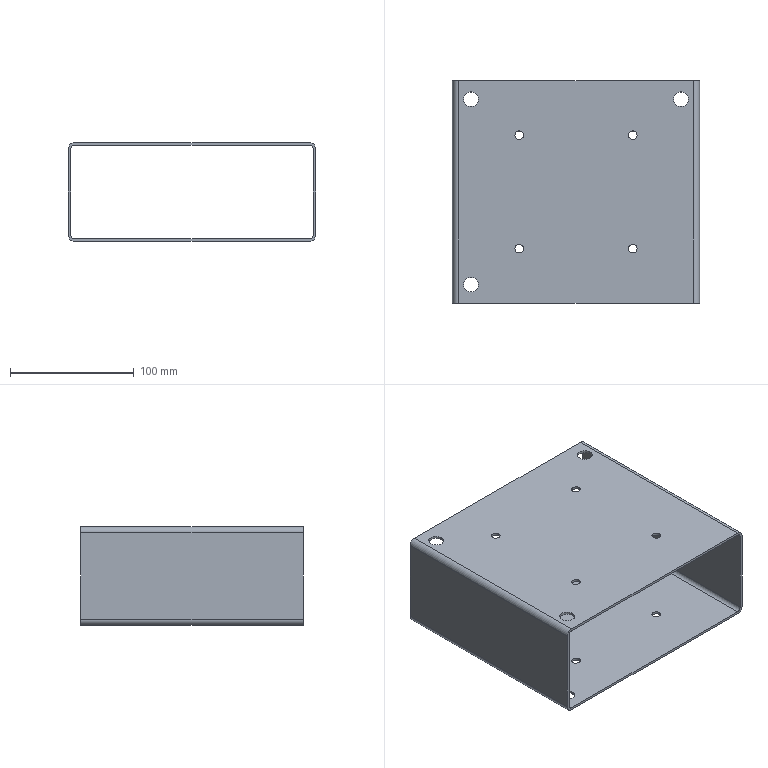Part | STEP file | Fixture seat bracket-market | 1 solid | 46 faces | box 200 x 180 x 80 mm | volume 194275 mm3 | cylinder 36 | plane 10 | commonest cylinder face diameters 7 x16 12 x12 6 x4 10 x4